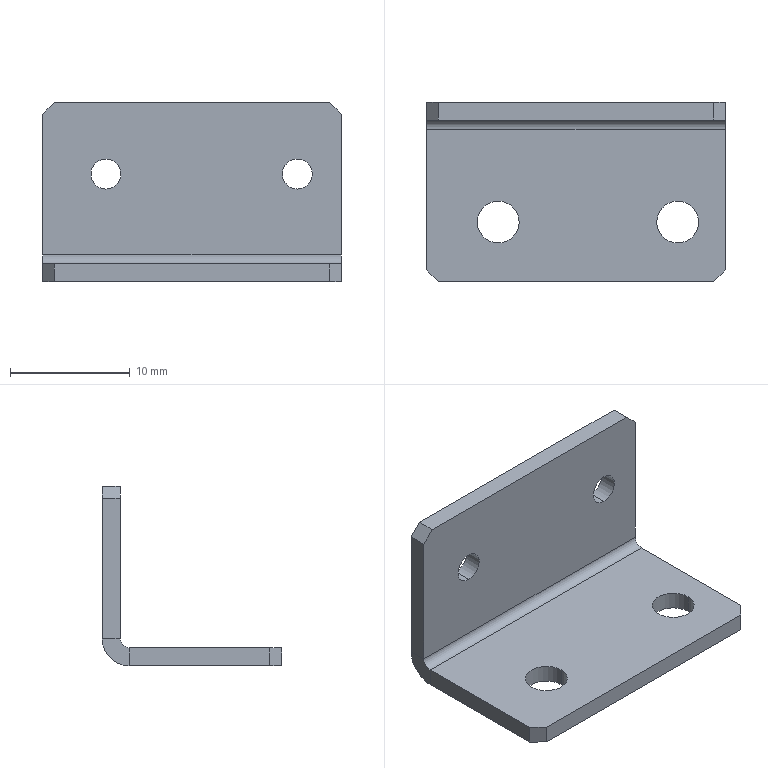Part | STEP file | PN_0029 BKT | 1 solid | 26 faces | box 25 x 15 x 15 mm | volume 998.233 mm3 | plane 16 | cylinder 10 | commonest cylinder face diameters 2.5 x4 3.5 x4 1.473 x1 4.473 x1